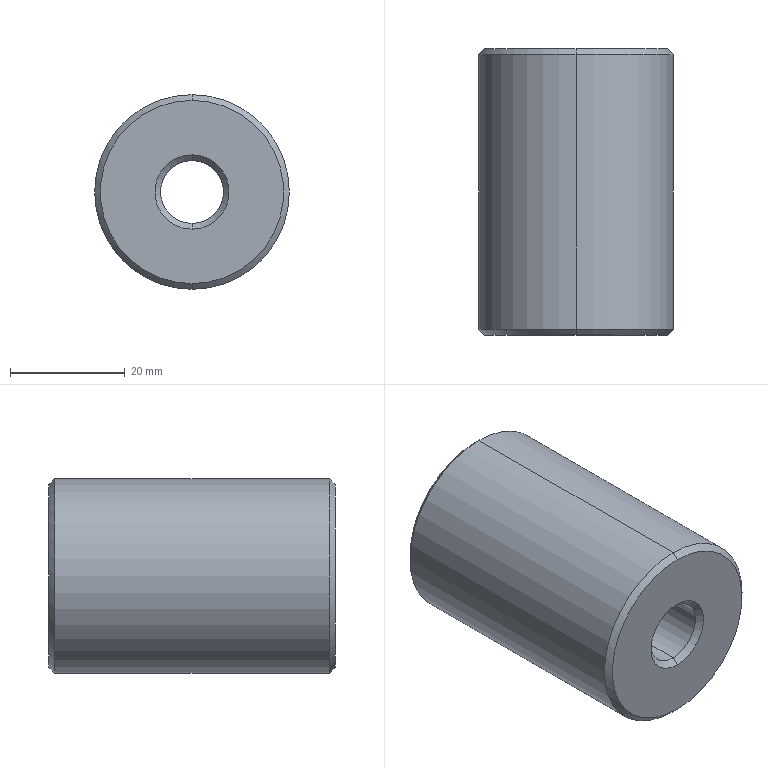Part | STEP file | Mould foot - Tower - 1 cav | 1 solid | 19 faces | box 34 x 50 x 34 mm | volume 31705 mm3 | cone 10 | cylinder 6 | plane 3 | commonest cylinder face diameters 11 x2 20 x2 34 x2
STEP:
#1=CARTESIAN_POINT('',(0.,0.,0.));
#2=DIRECTION('',(0.,0.,1.));
#3=DIRECTION('',(1.,0.,0.));
#4=AXIS2_PLACEMENT_3D('',#1,#2,#3);
#5=CARTESIAN_POINT('',(0.,9.,5.5));
#6=VERTEX_POINT('',#5);
#7=CARTESIAN_POINT('',(0.,10.,6.5));
#8=VERTEX_POINT('',#7);
#9=CARTESIAN_POINT('',(0.,10.,6.5));
#10=DIRECTION('',(0.,0.7071,0.7071));
#11=VECTOR('',#10,1.);
#12=LINE('',#9,#11);
#13=CARTESIAN_POINT('',(0.,10.,0.));
#14=DIRECTION('',(0.,1.,0.));
#15=DIRECTION('',(0.,0.,1.));
#16=AXIS2_PLACEMENT_3D('',#13,#14,#15);
#17=CONICAL_SURFACE('',#16,6.5,0.7854);
#18=CARTESIAN_POINT('',(6.283,0.));
#19=DIRECTION('',(0.,1.));
#20=VECTOR('',#19,1.);
#21=LINE('',#18,#20);
#22=(GEOMETRIC_REPRESENTATION_CONTEXT(2)PARAMETRIC_REPRESENTATION_CONTEXT()REPRESENTATION_CONTEXT('',''));
#23=DEFINITIONAL_REPRESENTATION('',(#21),#22);
#24=PCURVE('',#17,#23);
#25=CARTESIAN_POINT('',(0.,10.,0.));
#26=DIRECTION('',(0.,1.,0.));
#27=DIRECTION('',(0.,0.,1.));
#28=AXIS2_PLACEMENT_3D('',#25,#26,#27);
#29=CONICAL_SURFACE('',#28,6.5,0.7854);
#30=CARTESIAN_POINT('',(0.,0.));
#31=DIRECTION('',(0.,1.));
#32=VECTOR('',#31,1.);
#33=LINE('',#30,#32);
#34=(GEOMETRIC_REPRESENTATION_CONTEXT(2)PARAMETRIC_REPRESENTATION_CONTEXT()REPRESENTATION_CONTEXT('',''));
#35=DEFINITIONAL_REPRESENTATION('',(#33),#34);
#36=PCURVE('',#29,#35);
#37=SURFACE_CURVE('',#12,(#24,#36),.PCURVE_S1.);
#38=EDGE_CURVE('',#6,#8,#37,.T.);
#39=ORIENTED_EDGE('',*,*,#38,.T.);
#40=CARTESIAN_POINT('',(0.,10.,-6.5));
#41=VERTEX_POINT('',#40);
#42=CARTESIAN_POINT('',(0.,10.,0.));
#43=DIRECTION('',(0.,-1.,0.));
#44=DIRECTION('',(0.,0.,-1.));
#45=AXIS2_PLACEMENT_3D('',#42,#43,#44);
#46=CIRCLE('',#45,6.5);
#47=CARTESIAN_POINT('',(9.425,0.));
#48=DIRECTION('',(-1.,0.));
#49=VECTOR('',#48,1.);
#50=LINE('',#47,#49);
#51=(GEOMETRIC_REPRESENTATION_CONTEXT(2)PARAMETRIC_REPRESENTATION_CONTEXT()REPRESENTATION_CONTEXT('',''));
#52=DEFINITIONAL_REPRESENTATION('',(#50),#51);
#53=PCURVE('',#17,#52);
#54=CARTESIAN_POINT('',(0.,10.,-6.5));
#55=DIRECTION('',(0.,1.,0.));
#56=DIRECTION('',(0.,0.,1.));
#57=AXIS2_PLACEMENT_3D('',#54,#55,#56);
#58=PLANE('',#57);
#59=CARTESIAN_POINT('',(0.,0.));
#60=CARTESIAN_POINT('',(0.,11.258));
#61=CARTESIAN_POINT('',(9.75,5.629));
#62=CARTESIAN_POINT('',(19.5,0.));
#63=CARTESIAN_POINT('',(9.75,-5.629));
#64=CARTESIAN_POINT('',(0.,-11.258));
#65=CARTESIAN_POINT('',(0.,0.));
#66=(BOUNDED_CURVE()B_SPLINE_CURVE(2,(#59,#60,#61,#62,#63,#64,#65),.UNSPECIFIED.,.T.,.F.)B_SPLINE_CURVE_WITH_KNOTS((1,2,2,2,2,1),(-2.094,0.,2.094,4.189,6.283,8.378),.UNSPECIFIED.)CURVE()GEOMETRIC_REPRESENTATION_ITEM()RATIONAL_B_SPLINE_CURVE((1.,0.5,1.,0.5,1.,0.5,1.))REPRESENTATION_ITEM(''));
#67=(GEOMETRIC_REPRESENTATION_CONTEXT(2)PARAMETRIC_REPRESENTATION_CONTEXT()REPRESENTATION_CONTEXT('',''));
#68=DEFINITIONAL_REPRESENTATION('',(#66),#67);
#69=PCURVE('',#58,#68);
#70=SURFACE_CURVE('',#46,(#53,#69),.PCURVE_S1.);
#71=EDGE_CURVE('',#8,#41,#70,.T.);
#72=ORIENTED_EDGE('',*,*,#71,.T.);
#73=CARTESIAN_POINT('',(0.,9.,-5.5));
#74=VERTEX_POINT('',#73);
#75=CARTESIAN_POINT('',(0.,10.,-6.5));
#76=DIRECTION('',(0.,0.7071,-0.7071));
#77=VECTOR('',#76,1.);
#78=LINE('',#75,#77);
#79=CARTESIAN_POINT('',(3.142,0.));
#80=DIRECTION('',(0.,1.));
#81=VECTOR('',#80,1.);
#82=LINE('',#79,#81);
#83=(GEOMETRIC_REPRESENTATION_CONTEXT(2)PARAMETRIC_REPRESENTATION_CONTEXT()REPRESENTATION_CONTEXT('',''));
#84=DEFINITIONAL_REPRESENTATION('',(#82),#83);
#85=PCURVE('',#17,#84);
#86=CARTESIAN_POINT('',(3.142,0.));
#87=DIRECTION('',(0.,1.));
#88=VECTOR('',#87,1.);
#89=LINE('',#86,#88);
#90=(GEOMETRIC_REPRESENTATION_CONTEXT(2)PARAMETRIC_REPRESENTATION_CONTEXT()REPRESENTATION_CONTEXT('',''));
#91=DEFINITIONAL_REPRESENTATION('',(#89),#90);
#92=PCURVE('',#29,#91);
#93=SURFACE_CURVE('',#78,(#85,#92),.PCURVE_S1.);
#94=EDGE_CURVE('',#74,#41,#93,.T.);
#95=ORIENTED_EDGE('',*,*,#94,.F.);
#96=CARTESIAN_POINT('',(0.,9.,0.));
#97=DIRECTION('',(0.,-1.,0.));
#98=DIRECTION('',(0.,0.,-1.));
#99=AXIS2_PLACEMENT_3D('',#96,#97,#98);
#100=CIRCLE('',#99,5.5);
#101=CARTESIAN_POINT('',(9.425,-1.));
#102=DIRECTION('',(-1.,0.));
#103=VECTOR('',#102,1.);
#104=LINE('',#101,#103);
#105=(GEOMETRIC_REPRESENTATION_CONTEXT(2)PARAMETRIC_REPRESENTATION_CONTEXT()REPRESENTATION_CONTEXT('',''));
#106=DEFINITIONAL_REPRESENTATION('',(#104),#105);
#107=PCURVE('',#17,#106);
#108=CARTESIAN_POINT('',(0.,0.,0.));
#109=DIRECTION('',(0.,-1.,0.));
#110=DIRECTION('',(0.,0.,-1.));
#111=AXIS2_PLACEMENT_3D('',#108,#109,#110);
#112=CYLINDRICAL_SURFACE('',#111,5.5);
#113=CARTESIAN_POINT('',(0.,-9.));
#114=DIRECTION('',(1.,0.));
#115=VECTOR('',#114,1.);
#116=LINE('',#113,#115);
#117=(GEOMETRIC_REPRESENTATION_CONTEXT(2)PARAMETRIC_REPRESENTATION_CONTEXT()REPRESENTATION_CONTEXT('',''));
#118=DEFINITIONAL_REPRESENTATION('',(#116),#117);
#119=PCURVE('',#112,#118);
#120=SURFACE_CURVE('',#100,(#107,#119),.PCURVE_S1.);
#121=EDGE_CURVE('',#6,#74,#120,.T.);
#122=ORIENTED_EDGE('',*,*,#121,.F.);
#123=EDGE_LOOP('',(#39,#72,#95,#122));
#124=FACE_BOUND('',#123,.F.);
#125=ADVANCED_FACE('',(#124),#17,.F.);
#126=CARTESIAN_POINT('',(0.,1.,-5.5));
#127=VERTEX_POINT('',#126);
#128=CARTESIAN_POINT('',(0.,0.,-5.5));
#129=DIRECTION('',(0.,-1.,0.));
#130=VECTOR('',#129,1.);
#131=LINE('',#128,#130);
#132=CARTESIAN_POINT('',(6.283,0.));
#133=DIRECTION('',(0.,1.));
#134=VECTOR('',#133,1.);
#135=LINE('',#132,#134);
#136=(GEOMETRIC_REPRESENTATION_CONTEXT(2)PARAMETRIC_REPRESENTATION_CONTEXT()REPRESENTATION_CONTEXT('',''));
#137=DEFINITIONAL_REPRESENTATION('',(#135),#136);
#138=PCURVE('',#112,#137);
#139=CARTESIAN_POINT('',(0.,0.,0.));
#140=DIRECTION('',(0.,-1.,0.));
#141=DIRECTION('',(0.,0.,-1.));
#142=AXIS2_PLACEMENT_3D('',#139,#140,#141);
#143=CYLINDRICAL_SURFACE('',#142,5.5);
#144=CARTESIAN_POINT('',(0.,0.));
#145=DIRECTION('',(0.,1.));
#146=VECTOR('',#145,1.);
#147=LINE('',#144,#146);
#148=(GEOMETRIC_REPRESENTATION_CONTEXT(2)PARAMETRIC_REPRESENTATION_CONTEXT()REPRESENTATION_CONTEXT('',''));
#149=DEFINITIONAL_REPRESENTATION('',(#147),#148);
#150=PCURVE('',#143,#149);
#151=SURFACE_CURVE('',#131,(#138,#150),.PCURVE_S1.);
#152=EDGE_CURVE('',#74,#127,#151,.T.);
#153=ORIENTED_EDGE('',*,*,#152,.T.);
#154=CARTESIAN_POINT('',(0.,1.,5.5));
#155=VERTEX_POINT('',#154);
#156=CARTESIAN_POINT('',(0.,1.,0.));
#157=DIRECTION('',(0.,-1.,0.));
#158=DIRECTION('',(0.,0.,-1.));
#159=AXIS2_PLACEMENT_3D('',#156,#157,#158);
#160=CIRCLE('',#159,5.5);
#161=CARTESIAN_POINT('',(0.,-1.));
#162=DIRECTION('',(1.,0.));
#163=VECTOR('',#162,1.);
#164=LINE('',#161,#163);
#165=(GEOMETRIC_REPRESENTATION_CONTEXT(2)PARAMETRIC_REPRESENTATION_CONTEXT()REPRESENTATION_CONTEXT('',''));
#166=DEFINITIONAL_REPRESENTATION('',(#164),#165);
#167=PCURVE('',#112,#166);
#168=CARTESIAN_POINT('',(0.,1.,0.));
#169=DIRECTION('',(0.,-1.,0.));
#170=DIRECTION('',(0.,0.,-1.));
#171=AXIS2_PLACEMENT_3D('',#168,#169,#170);
#172=CONICAL_SURFACE('',#171,5.5,0.7854);
#173=CARTESIAN_POINT('',(0.,0.));
#174=DIRECTION('',(1.,0.));
#175=VECTOR('',#174,1.);
#176=LINE('',#173,#175);
#177=(GEOMETRIC_REPRESENTATION_CONTEXT(2)PARAMETRIC_REPRESENTATION_CONTEXT()REPRESENTATION_CONTEXT('',''));
#178=DEFINITIONAL_REPRESENTATION('',(#176),#177);
#179=PCURVE('',#172,#178);
#180=SURFACE_CURVE('',#160,(#167,#179),.PCURVE_S1.);
#181=EDGE_CURVE('',#155,#127,#180,.T.);
#182=ORIENTED_EDGE('',*,*,#181,.F.);
#183=CARTESIAN_POINT('',(0.,0.,5.5));
#184=DIRECTION('',(0.,-1.,0.));
#185=VECTOR('',#184,1.);
#186=LINE('',#183,#185);
#187=CARTESIAN_POINT('',(3.142,0.));
#188=DIRECTION('',(0.,1.));
#189=VECTOR('',#188,1.);
#190=LINE('',#187,#189);
#191=(GEOMETRIC_REPRESENTATION_CONTEXT(2)PARAMETRIC_REPRESENTATION_CONTEXT()REPRESENTATION_CONTEXT('',''));
#192=DEFINITIONAL_REPRESENTATION('',(#190),#191);
#193=PCURVE('',#112,#192);
#194=CARTESIAN_POINT('',(3.142,0.));
#195=DIRECTION('',(0.,1.));
#196=VECTOR('',#195,1.);
#197=LINE('',#194,#196);
#198=(GEOMETRIC_REPRESENTATION_CONTEXT(2)PARAMETRIC_REPRESENTATION_CONTEXT()REPRESENTATION_CONTEXT('',''));
#199=DEFINITIONAL_REPRESENTATION('',(#197),#198);
#200=PCURVE('',#143,#199);
#201=SURFACE_CURVE('',#186,(#193,#200),.PCURVE_S1.);
#202=EDGE_CURVE('',#6,#155,#201,.T.);
#203=ORIENTED_EDGE('',*,*,#202,.F.);
#204=ORIENTED_EDGE('',*,*,#121,.T.);
#205=EDGE_LOOP('',(#153,#182,#203,#204));
#206=FACE_BOUND('',#205,.F.);
#207=ADVANCED_FACE('',(#206),#112,.F.);
#208=CARTESIAN_POINT('',(0.,0.,-6.5));
#209=VERTEX_POINT('',#208);
#210=CARTESIAN_POINT('',(0.,1.,-5.5));
#211=DIRECTION('',(0.,-0.7071,-0.7071));
#212=VECTOR('',#211,1.);
#213=LINE('',#210,#212);
#214=CARTESIAN_POINT('',(6.283,0.));
#215=DIRECTION('',(0.,1.));
#216=VECTOR('',#215,1.);
#217=LINE('',#214,#216);
#218=(GEOMETRIC_REPRESENTATION_CONTEXT(2)PARAMETRIC_REPRESENTATION_CONTEXT()REPRESENTATION_CONTEXT('',''));
#219=DEFINITIONAL_REPRESENTATION('',(#217),#218);
#220=PCURVE('',#172,#219);
#221=CARTESIAN_POINT('',(0.,1.,0.));
#222=DIRECTION('',(0.,-1.,0.));
#223=DIRECTION('',(0.,0.,-1.));
#224=AXIS2_PLACEMENT_3D('',#221,#222,#223);
#225=CONICAL_SURFACE('',#224,5.5,0.7854);
#226=CARTESIAN_POINT('',(0.,0.));
#227=DIRECTION('',(0.,1.));
#228=VECTOR('',#227,1.);
#229=LINE('',#226,#228);
#230=(GEOMETRIC_REPRESENTATION_CONTEXT(2)PARAMETRIC_REPRESENTATION_CONTEXT()REPRESENTATION_CONTEXT('',''));
#231=DEFINITIONAL_REPRESENTATION('',(#229),#230);
#232=PCURVE('',#225,#231);
#233=SURFACE_CURVE('',#213,(#220,#232),.PCURVE_S1.);
#234=EDGE_CURVE('',#127,#209,#233,.T.);
#235=ORIENTED_EDGE('',*,*,#234,.T.);
#236=CARTESIAN_POINT('',(0.,0.,6.5));
#237=VERTEX_POINT('',#236);
#238=CARTESIAN_POINT('',(0.,0.,0.));
#239=DIRECTION('',(0.,-1.,0.));
#240=DIRECTION('',(0.,0.,-1.));
#241=AXIS2_PLACEMENT_3D('',#238,#239,#240);
#242=CIRCLE('',#241,6.5);
#243=CARTESIAN_POINT('',(0.,1.));
#244=DIRECTION('',(1.,0.));
#245=VECTOR('',#244,1.);
#246=LINE('',#243,#245);
#247=(GEOMETRIC_REPRESENTATION_CONTEXT(2)PARAMETRIC_REPRESENTATION_CONTEXT()REPRESENTATION_CONTEXT('',''));
#248=DEFINITIONAL_REPRESENTATION('',(#246),#247);
#249=PCURVE('',#172,#248);
#250=CARTESIAN_POINT('',(0.,0.,-16.));
#251=DIRECTION('',(0.,-1.,0.));
#252=DIRECTION('',(0.,0.,-1.));
#253=AXIS2_PLACEMENT_3D('',#250,#251,#252);
#254=PLANE('',#253);
#255=CARTESIAN_POINT('',(-16.,0.));
#256=DIRECTION('',(1.,0.));
#257=AXIS2_PLACEMENT_2D('',#255,#256);
#258=CIRCLE('',#257,6.5);
#259=(GEOMETRIC_REPRESENTATION_CONTEXT(2)PARAMETRIC_REPRESENTATION_CONTEXT()REPRESENTATION_CONTEXT('',''));
#260=DEFINITIONAL_REPRESENTATION('',(#258),#259);
#261=PCURVE('',#254,#260);
#262=SURFACE_CURVE('',#242,(#249,#261),.PCURVE_S1.);
#263=EDGE_CURVE('',#237,#209,#262,.T.);
#264=ORIENTED_EDGE('',*,*,#263,.F.);
#265=CARTESIAN_POINT('',(0.,1.,5.5));
#266=DIRECTION('',(0.,-0.7071,0.7071));
#267=VECTOR('',#266,1.);
#268=LINE('',#265,#267);
#269=CARTESIAN_POINT('',(3.142,0.));
#270=DIRECTION('',(0.,1.));
#271=VECTOR('',#270,1.);
#272=LINE('',#269,#271);
#273=(GEOMETRIC_REPRESENTATION_CONTEXT(2)PARAMETRIC_REPRESENTATION_CONTEXT()REPRESENTATION_CONTEXT('',''));
#274=DEFINITIONAL_REPRESENTATION('',(#272),#273);
#275=PCURVE('',#172,#274);
#276=CARTESIAN_POINT('',(3.142,0.));
#277=DIRECTION('',(0.,1.));
#278=VECTOR('',#277,1.);
#279=LINE('',#276,#278);
#280=(GEOMETRIC_REPRESENTATION_CONTEXT(2)PARAMETRIC_REPRESENTATION_CONTEXT()REPRESENTATION_CONTEXT('',''));
#281=DEFINITIONAL_REPRESENTATION('',(#279),#280);
#282=PCURVE('',#225,#281);
#283=SURFACE_CURVE('',#268,(#275,#282),.PCURVE_S1.);
#284=EDGE_CURVE('',#155,#237,#283,.T.);
#285=ORIENTED_EDGE('',*,*,#284,.F.);
#286=ORIENTED_EDGE('',*,*,#181,.T.);
#287=EDGE_LOOP('',(#235,#264,#285,#286));
#288=FACE_BOUND('',#287,.F.);
#289=ADVANCED_FACE('',(#288),#172,.F.);
#290=CARTESIAN_POINT('',(0.,0.,-16.));
#291=VERTEX_POINT('',#290);
#292=CARTESIAN_POINT('',(0.,0.,16.));
#293=VERTEX_POINT('',#292);
#294=CARTESIAN_POINT('',(0.,0.,0.));
#295=DIRECTION('',(0.,-1.,0.));
#296=DIRECTION('',(0.,0.,-1.));
#297=AXIS2_PLACEMENT_3D('',#294,#295,#296);
#298=CIRCLE('',#297,16.);
#299=CARTESIAN_POINT('',(0.,0.,0.));
#300=DIRECTION('',(0.,1.,0.));
#301=DIRECTION('',(0.,0.,1.));
#302=AXIS2_PLACEMENT_3D('',#299,#300,#301);
#303=CONICAL_SURFACE('',#302,16.,0.7854);
#304=CARTESIAN_POINT('',(3.142,0.));
#305=DIRECTION('',(-1.,0.));
#306=VECTOR('',#305,1.);
#307=LINE('',#304,#306);
#308=(GEOMETRIC_REPRESENTATION_CONTEXT(2)PARAMETRIC_REPRESENTATION_CONTEXT()REPRESENTATION_CONTEXT('',''));
#309=DEFINITIONAL_REPRESENTATION('',(#307),#308);
#310=PCURVE('',#303,#309);
#311=CARTESIAN_POINT('',(-16.,0.));
#312=DIRECTION('',(1.,0.));
#313=AXIS2_PLACEMENT_2D('',#311,#312);
#314=CIRCLE('',#313,16.);
#315=(GEOMETRIC_REPRESENTATION_CONTEXT(2)PARAMETRIC_REPRESENTATION_CONTEXT()REPRESENTATION_CONTEXT('',''));
#316=DEFINITIONAL_REPRESENTATION('',(#314),#315);
#317=PCURVE('',#254,#316);
#318=SURFACE_CURVE('',#298,(#310,#317),.PCURVE_S1.);
#319=EDGE_CURVE('',#291,#293,#318,.T.);
#320=ORIENTED_EDGE('',*,*,#319,.F.);
#321=CARTESIAN_POINT('',(0.,1.,-17.));
#322=VERTEX_POINT('',#321);
#323=CARTESIAN_POINT('',(0.,0.,-16.));
#324=DIRECTION('',(0.,0.7071,-0.7071));
#325=VECTOR('',#324,1.);
#326=LINE('',#323,#325);
#327=CARTESIAN_POINT('',(3.142,0.));
#328=DIRECTION('',(0.,1.));
#329=VECTOR('',#328,1.);
#330=LINE('',#327,#329);
#331=(GEOMETRIC_REPRESENTATION_CONTEXT(2)PARAMETRIC_REPRESENTATION_CONTEXT()REPRESENTATION_CONTEXT('',''));
#332=DEFINITIONAL_REPRESENTATION('',(#330),#331);
#333=PCURVE('',#303,#332);
#334=CARTESIAN_POINT('',(0.,0.,0.));
#335=DIRECTION('',(0.,1.,0.));
#336=DIRECTION('',(0.,0.,1.));
#337=AXIS2_PLACEMENT_3D('',#334,#335,#336);
#338=CONICAL_SURFACE('',#337,16.,0.7854);
#339=CARTESIAN_POINT('',(3.142,0.));
#340=DIRECTION('',(0.,1.));
#341=VECTOR('',#340,1.);
#342=LINE('',#339,#341);
#343=(GEOMETRIC_REPRESENTATION_CONTEXT(2)PARAMETRIC_REPRESENTATION_CONTEXT()REPRESENTATION_CONTEXT('',''));
#344=DEFINITIONAL_REPRESENTATION('',(#342),#343);
#345=PCURVE('',#338,#344);
#346=SURFACE_CURVE('',#326,(#333,#345),.PCURVE_S1.);
#347=EDGE_CURVE('',#291,#322,#346,.T.);
#348=ORIENTED_EDGE('',*,*,#347,.T.);
#349=CARTESIAN_POINT('',(0.,1.,17.));
#350=VERTEX_POINT('',#349);
#351=CARTESIAN_POINT('',(0.,1.,0.));
#352=DIRECTION('',(0.,-1.,0.));
#353=DIRECTION('',(0.,0.,-1.));
#354=AXIS2_PLACEMENT_3D('',#351,#352,#353);
#355=CIRCLE('',#354,17.);
#356=CARTESIAN_POINT('',(3.142,1.));
#357=DIRECTION('',(-1.,0.));
#358=VECTOR('',#357,1.);
#359=LINE('',#356,#358);
#360=(GEOMETRIC_REPRESENTATION_CONTEXT(2)PARAMETRIC_REPRESENTATION_CONTEXT()REPRESENTATION_CONTEXT('',''));
#361=DEFINITIONAL_REPRESENTATION('',(#359),#360);
#362=PCURVE('',#303,#361);
#363=CARTESIAN_POINT('',(0.,0.,0.));
#364=DIRECTION('',(0.,-1.,0.));
#365=DIRECTION('',(0.,0.,-1.));
#366=AXIS2_PLACEMENT_3D('',#363,#364,#365);
#367=CYLINDRICAL_SURFACE('',#366,17.);
#368=CARTESIAN_POINT('',(0.,-1.));
#369=DIRECTION('',(1.,0.));
#370=VECTOR('',#369,1.);
#371=LINE('',#368,#370);
#372=(GEOMETRIC_REPRESENTATION_CONTEXT(2)PARAMETRIC_REPRESENTATION_CONTEXT()REPRESENTATION_CONTEXT('',''));
#373=DEFINITIONAL_REPRESENTATION('',(#371),#372);
#374=PCURVE('',#367,#373);
#375=SURFACE_CURVE('',#355,(#362,#374),.PCURVE_S1.);
#376=EDGE_CURVE('',#322,#350,#375,.T.);
#377=ORIENTED_EDGE('',*,*,#376,.T.);
#378=CARTESIAN_POINT('',(0.,0.,16.));
#379=DIRECTION('',(0.,0.7071,0.7071));
#380=VECTOR('',#379,1.);
#381=LINE('',#378,#380);
#382=CARTESIAN_POINT('',(0.,0.));
#383=DIRECTION('',(0.,1.));
#384=VECTOR('',#383,1.);
#385=LINE('',#382,#384);
#386=(GEOMETRIC_REPRESENTATION_CONTEXT(2)PARAMETRIC_REPRESENTATION_CONTEXT()REPRESENTATION_CONTEXT('',''));
#387=DEFINITIONAL_REPRESENTATION('',(#385),#386);
#388=PCURVE('',#303,#387);
#389=CARTESIAN_POINT('',(6.283,0.));
#390=DIRECTION('',(0.,1.));
#391=VECTOR('',#390,1.);
#392=LINE('',#389,#391);
#393=(GEOMETRIC_REPRESENTATION_CONTEXT(2)PARAMETRIC_REPRESENTATION_CONTEXT()REPRESENTATION_CONTEXT('',''));
#394=DEFINITIONAL_REPRESENTATION('',(#392),#393);
#395=PCURVE('',#338,#394);
#396=SURFACE_CURVE('',#381,(#388,#395),.PCURVE_S1.);
#397=EDGE_CURVE('',#293,#350,#396,.T.);
#398=ORIENTED_EDGE('',*,*,#397,.F.);
#399=EDGE_LOOP('',(#320,#348,#377,#398));
#400=FACE_BOUND('',#399,.T.);
#401=ADVANCED_FACE('',(#400),#303,.T.);
#402=CARTESIAN_POINT('',(0.,49.,-17.));
#403=VERTEX_POINT('',#402);
#404=CARTESIAN_POINT('',(0.,49.,17.));
#405=VERTEX_POINT('',#404);
#406=CARTESIAN_POINT('',(0.,49.,0.));
#407=DIRECTION('',(0.,-1.,0.));
#408=DIRECTION('',(0.,0.,-1.));
#409=AXIS2_PLACEMENT_3D('',#406,#407,#408);
#410=CIRCLE('',#409,17.);
#411=CARTESIAN_POINT('',(0.,-49.));
#412=DIRECTION('',(1.,0.));
#413=VECTOR('',#412,1.);
#414=LINE('',#411,#413);
#415=(GEOMETRIC_REPRESENTATION_CONTEXT(2)PARAMETRIC_REPRESENTATION_CONTEXT()REPRESENTATION_CONTEXT('',''));
#416=DEFINITIONAL_REPRESENTATION('',(#414),#415);
#417=PCURVE('',#367,#416);
#418=CARTESIAN_POINT('',(0.,49.,0.));
#419=DIRECTION('',(0.,-1.,0.));
#420=DIRECTION('',(0.,0.,-1.));
#421=AXIS2_PLACEMENT_3D('',#418,#419,#420);
#422=CONICAL_SURFACE('',#421,17.,0.7854);
#423=CARTESIAN_POINT('',(0.,0.));
#424=DIRECTION('',(1.,0.));
#425=VECTOR('',#424,1.);
#426=LINE('',#423,#425);
#427=(GEOMETRIC_REPRESENTATION_CONTEXT(2)PARAMETRIC_REPRESENTATION_CONTEXT()REPRESENTATION_CONTEXT('',''));
#428=DEFINITIONAL_REPRESENTATION('',(#426),#427);
#429=PCURVE('',#422,#428);
#430=SURFACE_CURVE('',#410,(#417,#429),.PCURVE_S1.);
#431=EDGE_CURVE('',#403,#405,#430,.T.);
#432=ORIENTED_EDGE('',*,*,#431,.T.);
#433=CARTESIAN_POINT('',(0.,0.,17.));
#434=DIRECTION('',(0.,-1.,0.));
#435=VECTOR('',#434,1.);
#436=LINE('',#433,#435);
#437=CARTESIAN_POINT('',(3.142,0.));
#438=DIRECTION('',(0.,1.));
#439=VECTOR('',#438,1.);
#440=LINE('',#437,#439);
#441=(GEOMETRIC_REPRESENTATION_CONTEXT(2)PARAMETRIC_REPRESENTATION_CONTEXT()REPRESENTATION_CONTEXT('',''));
#442=DEFINITIONAL_REPRESENTATION('',(#440),#441);
#443=PCURVE('',#367,#442);
#444=CARTESIAN_POINT('',(0.,0.,0.));
#445=DIRECTION('',(0.,-1.,0.));
#446=DIRECTION('',(0.,0.,-1.));
#447=AXIS2_PLACEMENT_3D('',#444,#445,#446);
#448=CYLINDRICAL_SURFACE('',#447,17.);
#449=CARTESIAN_POINT('',(3.142,0.));
#450=DIRECTION('',(0.,1.));
#451=VECTOR('',#450,1.);
#452=LINE('',#449,#451);
#453=(GEOMETRIC_REPRESENTATION_CONTEXT(2)PARAMETRIC_REPRESENTATION_CONTEXT()REPRESENTATION_CONTEXT('',''));
#454=DEFINITIONAL_REPRESENTATION('',(#452),#453);
#455=PCURVE('',#448,#454);
#456=SURFACE_CURVE('',#436,(#443,#455),.PCURVE_S1.);
#457=EDGE_CURVE('',#405,#350,#456,.T.);
#458=ORIENTED_EDGE('',*,*,#457,.T.);
#459=ORIENTED_EDGE('',*,*,#376,.F.);
#460=CARTESIAN_POINT('',(0.,0.,-17.));
#461=DIRECTION('',(0.,-1.,0.));
#462=VECTOR('',#461,1.);
#463=LINE('',#460,#462);
#464=CARTESIAN_POINT('',(0.,0.));
#465=DIRECTION('',(0.,1.));
#466=VECTOR('',#465,1.);
#467=LINE('',#464,#466);
#468=(GEOMETRIC_REPRESENTATION_CONTEXT(2)PARAMETRIC_REPRESENTATION_CONTEXT()REPRESENTATION_CONTEXT('',''));
#469=DEFINITIONAL_REPRESENTATION('',(#467),#468);
#470=PCURVE('',#367,#469);
#471=CARTESIAN_POINT('',(6.283,0.));
#472=DIRECTION('',(0.,1.));
#473=VECTOR('',#472,1.);
#474=LINE('',#471,#473);
#475=(GEOMETRIC_REPRESENTATION_CONTEXT(2)PARAMETRIC_REPRESENTATION_CONTEXT()REPRESENTATION_CONTEXT('',''));
#476=DEFINITIONAL_REPRESENTATION('',(#474),#475);
#477=PCURVE('',#448,#476);
#478=SURFACE_CURVE('',#463,(#470,#477),.PCURVE_S1.);
#479=EDGE_CURVE('',#403,#322,#478,.T.);
#480=ORIENTED_EDGE('',*,*,#479,.F.);
#481=EDGE_LOOP('',(#432,#458,#459,#480));
#482=FACE_BOUND('',#481,.T.);
#483=ADVANCED_FACE('',(#482),#367,.T.);
#484=CARTESIAN_POINT('',(0.,50.,-16.));
#485=VERTEX_POINT('',#484);
#486=CARTESIAN_POINT('',(0.,50.,16.));
#487=VERTEX_POINT('',#486);
#488=CARTESIAN_POINT('',(0.,50.,0.));
#489=DIRECTION('',(0.,-1.,0.));
#490=DIRECTION('',(0.,0.,-1.));
#491=AXIS2_PLACEMENT_3D('',#488,#489,#490);
#492=CIRCLE('',#491,16.);
#493=CARTESIAN_POINT('',(0.,-1.));
#494=DIRECTION('',(1.,0.));
#495=VECTOR('',#494,1.);
#496=LINE('',#493,#495);
#497=(GEOMETRIC_REPRESENTATION_CONTEXT(2)PARAMETRIC_REPRESENTATION_CONTEXT()REPRESENTATION_CONTEXT('',''));
#498=DEFINITIONAL_REPRESENTATION('',(#496),#497);
#499=PCURVE('',#422,#498);
#500=CARTESIAN_POINT('',(0.,50.,-11.));
#501=DIRECTION('',(0.,1.,0.));
#502=DIRECTION('',(0.,0.,1.));
#503=AXIS2_PLACEMENT_3D('',#500,#501,#502);
#504=PLANE('',#503);
#505=CARTESIAN_POINT('',(-5.,0.));
#506=CARTESIAN_POINT('',(-5.,27.713));
#507=CARTESIAN_POINT('',(19.,13.856));
#508=CARTESIAN_POINT('',(43.,0.));
#509=CARTESIAN_POINT('',(19.,-13.856));
#510=CARTESIAN_POINT('',(-5.,-27.713));
#511=CARTESIAN_POINT('',(-5.,0.));
#512=(BOUNDED_CURVE()B_SPLINE_CURVE(2,(#505,#506,#507,#508,#509,#510,#511),.UNSPECIFIED.,.T.,.F.)B_SPLINE_CURVE_WITH_KNOTS((1,2,2,2,2,1),(-2.094,0.,2.094,4.189,6.283,8.378),.UNSPECIFIED.)CURVE()GEOMETRIC_REPRESENTATION_ITEM()RATIONAL_B_SPLINE_CURVE((1.,0.5,1.,0.5,1.,0.5,1.))REPRESENTATION_ITEM(''));
#513=(GEOMETRIC_REPRESENTATION_CONTEXT(2)PARAMETRIC_REPRESENTATION_CONTEXT()REPRESENTATION_CONTEXT('',''));
#514=DEFINITIONAL_REPRESENTATION('',(#512),#513);
#515=PCURVE('',#504,#514);
#516=SURFACE_CURVE('',#492,(#499,#515),.PCURVE_S1.);
#517=EDGE_CURVE('',#485,#487,#516,.T.);
#518=ORIENTED_EDGE('',*,*,#517,.T.);
#519=CARTESIAN_POINT('',(0.,49.,17.));
#520=DIRECTION('',(0.,-0.7071,0.7071));
#521=VECTOR('',#520,1.);
#522=LINE('',#519,#521);
#523=CARTESIAN_POINT('',(3.142,0.));
#524=DIRECTION('',(0.,1.));
#525=VECTOR('',#524,1.);
#526=LINE('',#523,#525);
#527=(GEOMETRIC_REPRESENTATION_CONTEXT(2)PARAMETRIC_REPRESENTATION_CONTEXT()REPRESENTATION_CONTEXT('',''));
#528=DEFINITIONAL_REPRESENTATION('',(#526),#527);
#529=PCURVE('',#422,#528);
#530=CARTESIAN_POINT('',(0.,49.,0.));
#531=DIRECTION('',(0.,-1.,0.));
#532=DIRECTION('',(0.,0.,-1.));
#533=AXIS2_PLACEMENT_3D('',#530,#531,#532);
#534=CONICAL_SURFACE('',#533,17.,0.7854);
#535=CARTESIAN_POINT('',(3.142,0.));
#536=DIRECTION('',(0.,1.));
#537=VECTOR('',#536,1.);
#538=LINE('',#535,#537);
#539=(GEOMETRIC_REPRESENTATION_CONTEXT(2)PARAMETRIC_REPRESENTATION_CONTEXT()REPRESENTATION_CONTEXT('',''));
#540=DEFINITIONAL_REPRESENTATION('',(#538),#539);
#541=PCURVE('',#534,#540);
#542=SURFACE_CURVE('',#522,(#529,#541),.PCURVE_S1.);
#543=EDGE_CURVE('',#487,#405,#542,.T.);
#544=ORIENTED_EDGE('',*,*,#543,.T.);
#545=ORIENTED_EDGE('',*,*,#431,.F.);
#546=CARTESIAN_POINT('',(0.,49.,-17.));
#547=DIRECTION('',(0.,-0.7071,-0.7071));
#548=VECTOR('',#547,1.);
#549=LINE('',#546,#548);
#550=CARTESIAN_POINT('',(0.,0.));
#551=DIRECTION('',(0.,1.));
#552=VECTOR('',#551,1.);
#553=LINE('',#550,#552);
#554=(GEOMETRIC_REPRESENTATION_CONTEXT(2)PARAMETRIC_REPRESENTATION_CONTEXT()REPRESENTATION_CONTEXT('',''));
#555=DEFINITIONAL_REPRESENTATION('',(#553),#554);
#556=PCURVE('',#422,#555);
#557=CARTESIAN_POINT('',(6.283,0.));
#558=DIRECTION('',(0.,1.));
#559=VECTOR('',#558,1.);
#560=LINE('',#557,#559);
#561=(GEOMETRIC_REPRESENTATION_CONTEXT(2)PARAMETRIC_REPRESENTATION_CONTEXT()REPRESENTATION_CONTEXT('',''));
#562=DEFINITIONAL_REPRESENTATION('',(#560),#561);
#563=PCURVE('',#534,#562);
#564=SURFACE_CURVE('',#549,(#556,#563),.PCURVE_S1.);
#565=EDGE_CURVE('',#485,#403,#564,.T.);
#566=ORIENTED_EDGE('',*,*,#565,.F.);
#567=EDGE_LOOP('',(#518,#544,#545,#566));
#568=FACE_BOUND('',#567,.T.);
#569=ADVANCED_FACE('',(#568),#422,.T.);
#570=CARTESIAN_POINT('',(0.,49.,10.));
#571=VERTEX_POINT('',#570);
#572=CARTESIAN_POINT('',(0.,50.,11.));
#573=VERTEX_POINT('',#572);
#574=CARTESIAN_POINT('',(0.,50.,11.));
#575=DIRECTION('',(0.,0.7071,0.7071));
#576=VECTOR('',#575,1.);
#577=LINE('',#574,#576);
#578=CARTESIAN_POINT('',(0.,50.,0.));
#579=DIRECTION('',(0.,1.,0.));
#580=DIRECTION('',(0.,0.,1.));
#581=AXIS2_PLACEMENT_3D('',#578,#579,#580);
#582=CONICAL_SURFACE('',#581,11.,0.7854);
#583=CARTESIAN_POINT('',(6.283,0.));
#584=DIRECTION('',(0.,1.));
#585=VECTOR('',#584,1.);
#586=LINE('',#583,#585);
#587=(GEOMETRIC_REPRESENTATION_CONTEXT(2)PARAMETRIC_REPRESENTATION_CONTEXT()REPRESENTATION_CONTEXT('',''));
#588=DEFINITIONAL_REPRESENTATION('',(#586),#587);
#589=PCURVE('',#582,#588);
#590=CARTESIAN_POINT('',(0.,50.,0.));
#591=DIRECTION('',(0.,1.,0.));
#592=DIRECTION('',(0.,0.,1.));
#593=AXIS2_PLACEMENT_3D('',#590,#591,#592);
#594=CONICAL_SURFACE('',#593,11.,0.7854);
#595=CARTESIAN_POINT('',(0.,0.));
#596=DIRECTION('',(0.,1.));
#597=VECTOR('',#596,1.);
#598=LINE('',#595,#597);
#599=(GEOMETRIC_REPRESENTATION_CONTEXT(2)PARAMETRIC_REPRESENTATION_CONTEXT()REPRESENTATION_CONTEXT('',''));
#600=DEFINITIONAL_REPRESENTATION('',(#598),#599);
#601=PCURVE('',#594,#600);
#602=SURFACE_CURVE('',#577,(#589,#601),.PCURVE_S1.);
#603=EDGE_CURVE('',#571,#573,#602,.T.);
#604=ORIENTED_EDGE('',*,*,#603,.T.);
#605=CARTESIAN_POINT('',(0.,50.,-11.));
#606=VERTEX_POINT('',#605);
#607=CARTESIAN_POINT('',(0.,50.,0.));
#608=DIRECTION('',(0.,-1.,0.));
#609=DIRECTION('',(0.,0.,-1.));
#610=AXIS2_PLACEMENT_3D('',#607,#608,#609);
#611=CIRCLE('',#610,11.);
#612=CARTESIAN_POINT('',(9.425,0.));
#613=DIRECTION('',(-1.,0.));
#614=VECTOR('',#613,1.);
#615=LINE('',#612,#614);
#616=(GEOMETRIC_REPRESENTATION_CONTEXT(2)PARAMETRIC_REPRESENTATION_CONTEXT()REPRESENTATION_CONTEXT('',''));
#617=DEFINITIONAL_REPRESENTATION('',(#615),#616);
#618=PCURVE('',#582,#617);
#619=CARTESIAN_POINT('',(0.,0.));
#620=CARTESIAN_POINT('',(0.,19.053));
#621=CARTESIAN_POINT('',(16.5,9.526));
#622=CARTESIAN_POINT('',(33.,0.));
#623=CARTESIAN_POINT('',(16.5,-9.526));
#624=CARTESIAN_POINT('',(0.,-19.053));
#625=CARTESIAN_POINT('',(0.,0.));
#626=(BOUNDED_CURVE()B_SPLINE_CURVE(2,(#619,#620,#621,#622,#623,#624,#625),.UNSPECIFIED.,.T.,.F.)B_SPLINE_CURVE_WITH_KNOTS((1,2,2,2,2,1),(-2.094,0.,2.094,4.189,6.283,8.378),.UNSPECIFIED.)CURVE()GEOMETRIC_REPRESENTATION_ITEM()RATIONAL_B_SPLINE_CURVE((1.,0.5,1.,0.5,1.,0.5,1.))REPRESENTATION_ITEM(''));
#627=(GEOMETRIC_REPRESENTATION_CONTEXT(2)PARAMETRIC_REPRESENTATION_CONTEXT()REPRESENTATION_CONTEXT('',''));
#628=DEFINITIONAL_REPRESENTATION('',(#626),#627);
#629=PCURVE('',#504,#628);
#630=SURFACE_CURVE('',#611,(#618,#629),.PCURVE_S1.);
#631=EDGE_CURVE('',#573,#606,#630,.T.);
#632=ORIENTED_EDGE('',*,*,#631,.T.);
#633=CARTESIAN_POINT('',(0.,49.,-10.));
#634=VERTEX_POINT('',#633);
#635=CARTESIAN_POINT('',(0.,50.,-11.));
#636=DIRECTION('',(0.,0.7071,-0.7071));
#637=VECTOR('',#636,1.);
#638=LINE('',#635,#637);
#639=CARTESIAN_POINT('',(3.142,0.));
#640=DIRECTION('',(0.,1.));
#641=VECTOR('',#640,1.);
#642=LINE('',#639,#641);
#643=(GEOMETRIC_REPRESENTATION_CONTEXT(2)PARAMETRIC_REPRESENTATION_CONTEXT()REPRESENTATION_CONTEXT('',''));
#644=DEFINITIONAL_REPRESENTATION('',(#642),#643);
#645=PCURVE('',#582,#644);
#646=CARTESIAN_POINT('',(3.142,0.));
#647=DIRECTION('',(0.,1.));
#648=VECTOR('',#647,1.);
#649=LINE('',#646,#648);
#650=(GEOMETRIC_REPRESENTATION_CONTEXT(2)PARAMETRIC_REPRESENTATION_CONTEXT()REPRESENTATION_CONTEXT('',''));
#651=DEFINITIONAL_REPRESENTATION('',(#649),#650);
#652=PCURVE('',#594,#651);
#653=SURFACE_CURVE('',#638,(#645,#652),.PCURVE_S1.);
#654=EDGE_CURVE('',#634,#606,#653,.T.);
#655=ORIENTED_EDGE('',*,*,#654,.F.);
#656=CARTESIAN_POINT('',(0.,49.,0.));
#657=DIRECTION('',(0.,-1.,0.));
#658=DIRECTION('',(0.,0.,-1.));
#659=AXIS2_PLACEMENT_3D('',#656,#657,#658);
#660=CIRCLE('',#659,10.);
#661=CARTESIAN_POINT('',(9.425,-1.));
#662=DIRECTION('',(-1.,0.));
#663=VECTOR('',#662,1.);
#664=LINE('',#661,#663);
#665=(GEOMETRIC_REPRESENTATION_CONTEXT(2)PARAMETRIC_REPRESENTATION_CONTEXT()REPRESENTATION_CONTEXT('',''));
#666=DEFINITIONAL_REPRESENTATION('',(#664),#665);
#667=PCURVE('',#582,#666);
#668=CARTESIAN_POINT('',(0.,0.,0.));
#669=DIRECTION('',(0.,-1.,0.));
#670=DIRECTION('',(0.,0.,-1.));
#671=AXIS2_PLACEMENT_3D('',#668,#669,#670);
#672=CYLINDRICAL_SURFACE('',#671,10.);
#673=CARTESIAN_POINT('',(0.,-49.));
#674=DIRECTION('',(1.,0.));
#675=VECTOR('',#674,1.);
#676=LINE('',#673,#675);
#677=(GEOMETRIC_REPRESENTATION_CONTEXT(2)PARAMETRIC_REPRESENTATION_CONTEXT()REPRESENTATION_CONTEXT('',''));
#678=DEFINITIONAL_REPRESENTATION('',(#676),#677);
#679=PCURVE('',#672,#678);
#680=SURFACE_CURVE('',#660,(#667,#679),.PCURVE_S1.);
#681=EDGE_CURVE('',#571,#634,#680,.T.);
#682=ORIENTED_EDGE('',*,*,#681,.F.);
#683=EDGE_LOOP('',(#604,#632,#655,#682));
#684=FACE_BOUND('',#683,.F.);
#685=ADVANCED_FACE('',(#684),#582,.F.);
#686=CARTESIAN_POINT('',(0.,10.,-10.));
#687=VERTEX_POINT('',#686);
#688=CARTESIAN_POINT('',(0.,0.,-10.));
#689=DIRECTION('',(0.,-1.,0.));
#690=VECTOR('',#689,1.);
#691=LINE('',#688,#690);
#692=CARTESIAN_POINT('',(6.283,0.));
#693=DIRECTION('',(0.,1.));
#694=VECTOR('',#693,1.);
#695=LINE('',#692,#694);
#696=(GEOMETRIC_REPRESENTATION_CONTEXT(2)PARAMETRIC_REPRESENTATION_CONTEXT()REPRESENTATION_CONTEXT('',''));
#697=DEFINITIONAL_REPRESENTATION('',(#695),#696);
#698=PCURVE('',#672,#697);
#699=CARTESIAN_POINT('',(0.,0.,0.));
#700=DIRECTION('',(0.,-1.,0.));
#701=DIRECTION('',(0.,0.,-1.));
#702=AXIS2_PLACEMENT_3D('',#699,#700,#701);
#703=CYLINDRICAL_SURFACE('',#702,10.);
#704=CARTESIAN_POINT('',(0.,0.));
#705=DIRECTION('',(0.,1.));
#706=VECTOR('',#705,1.);
#707=LINE('',#704,#706);
#708=(GEOMETRIC_REPRESENTATION_CONTEXT(2)PARAMETRIC_REPRESENTATION_CONTEXT()REPRESENTATION_CONTEXT('',''));
#709=DEFINITIONAL_REPRESENTATION('',(#707),#708);
#710=PCURVE('',#703,#709);
#711=SURFACE_CURVE('',#691,(#698,#710),.PCURVE_S1.);
#712=EDGE_CURVE('',#634,#687,#711,.T.);
#713=ORIENTED_EDGE('',*,*,#712,.T.);
#714=CARTESIAN_POINT('',(0.,10.,10.));
#715=VERTEX_POINT('',#714);
#716=CARTESIAN_POINT('',(0.,10.,0.));
#717=DIRECTION('',(0.,-1.,0.));
#718=DIRECTION('',(0.,0.,-1.));
#719=AXIS2_PLACEMENT_3D('',#716,#717,#718);
#720=CIRCLE('',#719,10.);
#721=CARTESIAN_POINT('',(0.,-10.));
#722=DIRECTION('',(1.,0.));
#723=VECTOR('',#722,1.);
#724=LINE('',#721,#723);
#725=(GEOMETRIC_REPRESENTATION_CONTEXT(2)PARAMETRIC_REPRESENTATION_CONTEXT()REPRESENTATION_CONTEXT('',''));
#726=DEFINITIONAL_REPRESENTATION('',(#724),#725);
#727=PCURVE('',#672,#726);
#728=CARTESIAN_POINT('',(-3.5,0.));
#729=CARTESIAN_POINT('',(-3.5,17.321));
#730=CARTESIAN_POINT('',(11.5,8.66));
#731=CARTESIAN_POINT('',(26.5,0.));
#732=CARTESIAN_POINT('',(11.5,-8.66));
#733=CARTESIAN_POINT('',(-3.5,-17.321));
#734=CARTESIAN_POINT('',(-3.5,0.));
#735=(BOUNDED_CURVE()B_SPLINE_CURVE(2,(#728,#729,#730,#731,#732,#733,#734),.UNSPECIFIED.,.T.,.F.)B_SPLINE_CURVE_WITH_KNOTS((1,2,2,2,2,1),(-2.094,0.,2.094,4.189,6.283,8.378),.UNSPECIFIED.)CURVE()GEOMETRIC_REPRESENTATION_ITEM()RATIONAL_B_SPLINE_CURVE((1.,0.5,1.,0.5,1.,0.5,1.))REPRESENTATION_ITEM(''));
#736=(GEOMETRIC_REPRESENTATION_CONTEXT(2)PARAMETRIC_REPRESENTATION_CONTEXT()REPRESENTATION_CONTEXT('',''));
#737=DEFINITIONAL_REPRESENTATION('',(#735),#736);
#738=PCURVE('',#58,#737);
#739=SURFACE_CURVE('',#720,(#727,#738),.PCURVE_S1.);
#740=EDGE_CURVE('',#715,#687,#739,.T.);
#741=ORIENTED_EDGE('',*,*,#740,.F.);
#742=CARTESIAN_POINT('',(0.,0.,10.));
#743=DIRECTION('',(0.,-1.,0.));
#744=VECTOR('',#743,1.);
#745=LINE('',#742,#744);
#746=CARTESIAN_POINT('',(3.142,0.));
#747=DIRECTION('',(0.,1.));
#748=VECTOR('',#747,1.);
#749=LINE('',#746,#748);
#750=(GEOMETRIC_REPRESENTATION_CONTEXT(2)PARAMETRIC_REPRESENTATION_CONTEXT()REPRESENTATION_CONTEXT('',''));
#751=DEFINITIONAL_REPRESENTATION('',(#749),#750);
#752=PCURVE('',#672,#751);
#753=CARTESIAN_POINT('',(3.142,0.));
#754=DIRECTION('',(0.,1.));
#755=VECTOR('',#754,1.);
#756=LINE('',#753,#755);
#757=(GEOMETRIC_REPRESENTATION_CONTEXT(2)PARAMETRIC_REPRESENTATION_CONTEXT()REPRESENTATION_CONTEXT('',''));
#758=DEFINITIONAL_REPRESENTATION('',(#756),#757);
#759=PCURVE('',#703,#758);
#760=SURFACE_CURVE('',#745,(#752,#759),.PCURVE_S1.);
#761=EDGE_CURVE('',#571,#715,#760,.T.);
#762=ORIENTED_EDGE('',*,*,#761,.F.);
#763=ORIENTED_EDGE('',*,*,#681,.T.);
#764=EDGE_LOOP('',(#713,#741,#762,#763));
#765=FACE_BOUND('',#764,.F.);
#766=ADVANCED_FACE('',(#765),#672,.F.);
#767=CARTESIAN_POINT('',(0.,10.,0.));
#768=DIRECTION('',(0.,-1.,0.));
#769=DIRECTION('',(0.,0.,-1.));
#770=AXIS2_PLACEMENT_3D('',#767,#768,#769);
#771=CIRCLE('',#770,10.);
#772=CARTESIAN_POINT('',(0.,-10.));
#773=DIRECTION('',(1.,0.));
#774=VECTOR('',#773,1.);
#775=LINE('',#772,#774);
#776=(GEOMETRIC_REPRESENTATION_CONTEXT(2)PARAMETRIC_REPRESENTATION_CONTEXT()REPRESENTATION_CONTEXT('',''));
#777=DEFINITIONAL_REPRESENTATION('',(#775),#776);
#778=PCURVE('',#703,#777);
#779=CARTESIAN_POINT('',(-3.5,0.));
#780=CARTESIAN_POINT('',(-3.5,17.321));
#781=CARTESIAN_POINT('',(11.5,8.66));
#782=CARTESIAN_POINT('',(26.5,0.));
#783=CARTESIAN_POINT('',(11.5,-8.66));
#784=CARTESIAN_POINT('',(-3.5,-17.321));
#785=CARTESIAN_POINT('',(-3.5,0.));
#786=(BOUNDED_CURVE()B_SPLINE_CURVE(2,(#779,#780,#781,#782,#783,#784,#785),.UNSPECIFIED.,.T.,.F.)B_SPLINE_CURVE_WITH_KNOTS((1,2,2,2,2,1),(-2.094,0.,2.094,4.189,6.283,8.378),.UNSPECIFIED.)CURVE()GEOMETRIC_REPRESENTATION_ITEM()RATIONAL_B_SPLINE_CURVE((1.,0.5,1.,0.5,1.,0.5,1.))REPRESENTATION_ITEM(''));
#787=(GEOMETRIC_REPRESENTATION_CONTEXT(2)PARAMETRIC_REPRESENTATION_CONTEXT()REPRESENTATION_CONTEXT('',''));
#788=DEFINITIONAL_REPRESENTATION('',(#786),#787);
#789=PCURVE('',#58,#788);
#790=SURFACE_CURVE('',#771,(#778,#789),.PCURVE_S1.);
#791=EDGE_CURVE('',#687,#715,#790,.T.);
#792=ORIENTED_EDGE('',*,*,#791,.F.);
#793=ORIENTED_EDGE('',*,*,#712,.F.);
#794=CARTESIAN_POINT('',(0.,49.,0.));
#795=DIRECTION('',(0.,-1.,0.));
#796=DIRECTION('',(0.,0.,-1.));
#797=AXIS2_PLACEMENT_3D('',#794,#795,#796);
#798=CIRCLE('',#797,10.);
#799=CARTESIAN_POINT('',(0.,-49.));
#800=DIRECTION('',(1.,0.));
#801=VECTOR('',#800,1.);
#802=LINE('',#799,#801);
#803=(GEOMETRIC_REPRESENTATION_CONTEXT(2)PARAMETRIC_REPRESENTATION_CONTEXT()REPRESENTATION_CONTEXT('',''));
#804=DEFINITIONAL_REPRESENTATION('',(#802),#803);
#805=PCURVE('',#703,#804);
#806=CARTESIAN_POINT('',(3.142,-1.));
#807=DIRECTION('',(-1.,0.));
#808=VECTOR('',#807,1.);
#809=LINE('',#806,#808);
#810=(GEOMETRIC_REPRESENTATION_CONTEXT(2)PARAMETRIC_REPRESENTATION_CONTEXT()REPRESENTATION_CONTEXT('',''));
#811=DEFINITIONAL_REPRESENTATION('',(#809),#810);
#812=PCURVE('',#594,#811);
#813=SURFACE_CURVE('',#798,(#805,#812),.PCURVE_S1.);
#814=EDGE_CURVE('',#634,#571,#813,.T.);
#815=ORIENTED_EDGE('',*,*,#814,.T.);
#816=ORIENTED_EDGE('',*,*,#761,.T.);
#817=EDGE_LOOP('',(#792,#793,#815,#816));
#818=FACE_BOUND('',#817,.F.);
#819=ADVANCED_FACE('',(#818),#703,.F.);
#820=CARTESIAN_POINT('',(0.,50.,0.));
#821=DIRECTION('',(0.,-1.,0.));
#822=DIRECTION('',(0.,0.,-1.));
#823=AXIS2_PLACEMENT_3D('',#820,#821,#822);
#824=CIRCLE('',#823,11.);
#825=CARTESIAN_POINT('',(3.142,0.));
#826=DIRECTION('',(-1.,0.));
#827=VECTOR('',#826,1.);
#828=LINE('',#825,#827);
#829=(GEOMETRIC_REPRESENTATION_CONTEXT(2)PARAMETRIC_REPRESENTATION_CONTEXT()REPRESENTATION_CONTEXT('',''));
#830=DEFINITIONAL_REPRESENTATION('',(#828),#829);
#831=PCURVE('',#594,#830);
#832=CARTESIAN_POINT('',(0.,0.));
#833=CARTESIAN_POINT('',(0.,19.053));
#834=CARTESIAN_POINT('',(16.5,9.526));
#835=CARTESIAN_POINT('',(33.,0.));
#836=CARTESIAN_POINT('',(16.5,-9.526));
#837=CARTESIAN_POINT('',(0.,-19.053));
#838=CARTESIAN_POINT('',(0.,0.));
#839=(BOUNDED_CURVE()B_SPLINE_CURVE(2,(#832,#833,#834,#835,#836,#837,#838),.UNSPECIFIED.,.T.,.F.)B_SPLINE_CURVE_WITH_KNOTS((1,2,2,2,2,1),(-2.094,0.,2.094,4.189,6.283,8.378),.UNSPECIFIED.)CURVE()GEOMETRIC_REPRESENTATION_ITEM()RATIONAL_B_SPLINE_CURVE((1.,0.5,1.,0.5,1.,0.5,1.))REPRESENTATION_ITEM(''));
#840=(GEOMETRIC_REPRESENTATION_CONTEXT(2)PARAMETRIC_REPRESENTATION_CONTEXT()REPRESENTATION_CONTEXT('',''));
#841=DEFINITIONAL_REPRESENTATION('',(#839),#840);
#842=PCURVE('',#504,#841);
#843=SURFACE_CURVE('',#824,(#831,#842),.PCURVE_S1.);
#844=EDGE_CURVE('',#606,#573,#843,.T.);
#845=ORIENTED_EDGE('',*,*,#844,.T.);
#846=ORIENTED_EDGE('',*,*,#603,.F.);
#847=ORIENTED_EDGE('',*,*,#814,.F.);
#848=ORIENTED_EDGE('',*,*,#654,.T.);
#849=EDGE_LOOP('',(#845,#846,#847,#848));
#850=FACE_BOUND('',#849,.F.);
#851=ADVANCED_FACE('',(#850),#594,.F.);
#852=ORIENTED_EDGE('',*,*,#631,.T.);
#853=ORIENTED_EDGE('',*,*,#844,.T.);
#854=EDGE_LOOP('',(#852,#853));
#855=FACE_BOUND('',#854,.T.);
#856=ORIENTED_EDGE('',*,*,#517,.F.);
#857=CARTESIAN_POINT('',(0.,50.,0.));
#858=DIRECTION('',(0.,-1.,0.));
#859=DIRECTION('',(0.,0.,-1.));
#860=AXIS2_PLACEMENT_3D('',#857,#858,#859);
#861=CIRCLE('',#860,16.);
#862=CARTESIAN_POINT('',(-5.,0.));
#863=CARTESIAN_POINT('',(-5.,27.713));
#864=CARTESIAN_POINT('',(19.,13.856));
#865=CARTESIAN_POINT('',(43.,0.));
#866=CARTESIAN_POINT('',(19.,-13.856));
#867=CARTESIAN_POINT('',(-5.,-27.713));
#868=CARTESIAN_POINT('',(-5.,0.));
#869=(BOUNDED_CURVE()B_SPLINE_CURVE(2,(#862,#863,#864,#865,#866,#867,#868),.UNSPECIFIED.,.T.,.F.)B_SPLINE_CURVE_WITH_KNOTS((1,2,2,2,2,1),(-2.094,0.,2.094,4.189,6.283,8.378),.UNSPECIFIED.)CURVE()GEOMETRIC_REPRESENTATION_ITEM()RATIONAL_B_SPLINE_CURVE((1.,0.5,1.,0.5,1.,0.5,1.))REPRESENTATION_ITEM(''));
#870=(GEOMETRIC_REPRESENTATION_CONTEXT(2)PARAMETRIC_REPRESENTATION_CONTEXT()REPRESENTATION_CONTEXT('',''));
#871=DEFINITIONAL_REPRESENTATION('',(#869),#870);
#872=PCURVE('',#504,#871);
#873=CARTESIAN_POINT('',(0.,-1.));
#874=DIRECTION('',(1.,0.));
#875=VECTOR('',#874,1.);
#876=LINE('',#873,#875);
#877=(GEOMETRIC_REPRESENTATION_CONTEXT(2)PARAMETRIC_REPRESENTATION_CONTEXT()REPRESENTATION_CONTEXT('',''));
#878=DEFINITIONAL_REPRESENTATION('',(#876),#877);
#879=PCURVE('',#534,#878);
#880=SURFACE_CURVE('',#861,(#872,#879),.PCURVE_S1.);
#881=EDGE_CURVE('',#487,#485,#880,.T.);
#882=ORIENTED_EDGE('',*,*,#881,.F.);
#883=EDGE_LOOP('',(#856,#882));
#884=FACE_BOUND('',#883,.T.);
#885=ADVANCED_FACE('',(#855,#884),#504,.T.);
#886=ORIENTED_EDGE('',*,*,#543,.F.);
#887=ORIENTED_EDGE('',*,*,#881,.T.);
#888=ORIENTED_EDGE('',*,*,#565,.T.);
#889=CARTESIAN_POINT('',(0.,49.,0.));
#890=DIRECTION('',(0.,-1.,0.));
#891=DIRECTION('',(0.,0.,-1.));
#892=AXIS2_PLACEMENT_3D('',#889,#890,#891);
#893=CIRCLE('',#892,17.);
#894=CARTESIAN_POINT('',(0.,0.));
#895=DIRECTION('',(1.,0.));
#896=VECTOR('',#895,1.);
#897=LINE('',#894,#896);
#898=(GEOMETRIC_REPRESENTATION_CONTEXT(2)PARAMETRIC_REPRESENTATION_CONTEXT()REPRESENTATION_CONTEXT('',''));
#899=DEFINITIONAL_REPRESENTATION('',(#897),#898);
#900=PCURVE('',#534,#899);
#901=CARTESIAN_POINT('',(0.,-49.));
#902=DIRECTION('',(1.,0.));
#903=VECTOR('',#902,1.);
#904=LINE('',#901,#903);
#905=(GEOMETRIC_REPRESENTATION_CONTEXT(2)PARAMETRIC_REPRESENTATION_CONTEXT()REPRESENTATION_CONTEXT('',''));
#906=DEFINITIONAL_REPRESENTATION('',(#904),#905);
#907=PCURVE('',#448,#906);
#908=SURFACE_CURVE('',#893,(#900,#907),.PCURVE_S1.);
#909=EDGE_CURVE('',#405,#403,#908,.T.);
#910=ORIENTED_EDGE('',*,*,#909,.F.);
#911=EDGE_LOOP('',(#886,#887,#888,#910));
#912=FACE_BOUND('',#911,.T.);
#913=ADVANCED_FACE('',(#912),#534,.T.);
#914=ORIENTED_EDGE('',*,*,#457,.F.);
#915=ORIENTED_EDGE('',*,*,#909,.T.);
#916=ORIENTED_EDGE('',*,*,#479,.T.);
#917=CARTESIAN_POINT('',(0.,1.,0.));
#918=DIRECTION('',(0.,-1.,0.));
#919=DIRECTION('',(0.,0.,-1.));
#920=AXIS2_PLACEMENT_3D('',#917,#918,#919);
#921=CIRCLE('',#920,17.);
#922=CARTESIAN_POINT('',(0.,-1.));
#923=DIRECTION('',(1.,0.));
#924=VECTOR('',#923,1.);
#925=LINE('',#922,#924);
#926=(GEOMETRIC_REPRESENTATION_CONTEXT(2)PARAMETRIC_REPRESENTATION_CONTEXT()REPRESENTATION_CONTEXT('',''));
#927=DEFINITIONAL_REPRESENTATION('',(#925),#926);
#928=PCURVE('',#448,#927);
#929=CARTESIAN_POINT('',(9.425,1.));
#930=DIRECTION('',(-1.,0.));
#931=VECTOR('',#930,1.);
#932=LINE('',#929,#931);
#933=(GEOMETRIC_REPRESENTATION_CONTEXT(2)PARAMETRIC_REPRESENTATION_CONTEXT()REPRESENTATION_CONTEXT('',''));
#934=DEFINITIONAL_REPRESENTATION('',(#932),#933);
#935=PCURVE('',#338,#934);
#936=SURFACE_CURVE('',#921,(#928,#935),.PCURVE_S1.);
#937=EDGE_CURVE('',#350,#322,#936,.T.);
#938=ORIENTED_EDGE('',*,*,#937,.F.);
#939=EDGE_LOOP('',(#914,#915,#916,#938));
#940=FACE_BOUND('',#939,.T.);
#941=ADVANCED_FACE('',(#940),#448,.T.);
#942=ORIENTED_EDGE('',*,*,#347,.F.);
#943=CARTESIAN_POINT('',(0.,0.,0.));
#944=DIRECTION('',(0.,-1.,0.));
#945=DIRECTION('',(0.,0.,-1.));
#946=AXIS2_PLACEMENT_3D('',#943,#944,#945);
#947=CIRCLE('',#946,16.);
#948=CARTESIAN_POINT('',(9.425,0.));
#949=DIRECTION('',(-1.,0.));
#950=VECTOR('',#949,1.);
#951=LINE('',#948,#950);
#952=(GEOMETRIC_REPRESENTATION_CONTEXT(2)PARAMETRIC_REPRESENTATION_CONTEXT()REPRESENTATION_CONTEXT('',''));
#953=DEFINITIONAL_REPRESENTATION('',(#951),#952);
#954=PCURVE('',#338,#953);
#955=CARTESIAN_POINT('',(-16.,0.));
#956=DIRECTION('',(1.,0.));
#957=AXIS2_PLACEMENT_2D('',#955,#956);
#958=CIRCLE('',#957,16.);
#959=(GEOMETRIC_REPRESENTATION_CONTEXT(2)PARAMETRIC_REPRESENTATION_CONTEXT()REPRESENTATION_CONTEXT('',''));
#960=DEFINITIONAL_REPRESENTATION('',(#958),#959);
#961=PCURVE('',#254,#960);
#962=SURFACE_CURVE('',#947,(#954,#961),.PCURVE_S1.);
#963=EDGE_CURVE('',#293,#291,#962,.T.);
#964=ORIENTED_EDGE('',*,*,#963,.F.);
#965=ORIENTED_EDGE('',*,*,#397,.T.);
#966=ORIENTED_EDGE('',*,*,#937,.T.);
#967=EDGE_LOOP('',(#942,#964,#965,#966));
#968=FACE_BOUND('',#967,.T.);
#969=ADVANCED_FACE('',(#968),#338,.T.);
#970=ORIENTED_EDGE('',*,*,#963,.T.);
#971=ORIENTED_EDGE('',*,*,#319,.T.);
#972=EDGE_LOOP('',(#970,#971));
#973=FACE_BOUND('',#972,.T.);
#974=CARTESIAN_POINT('',(0.,0.,0.));
#975=DIRECTION('',(0.,-1.,0.));
#976=DIRECTION('',(0.,0.,-1.));
#977=AXIS2_PLACEMENT_3D('',#974,#975,#976);
#978=CIRCLE('',#977,6.5);
#979=CARTESIAN_POINT('',(-16.,0.));
#980=DIRECTION('',(1.,0.));
#981=AXIS2_PLACEMENT_2D('',#979,#980);
#982=CIRCLE('',#981,6.5);
#983=(GEOMETRIC_REPRESENTATION_CONTEXT(2)PARAMETRIC_REPRESENTATION_CONTEXT()REPRESENTATION_CONTEXT('',''));
#984=DEFINITIONAL_REPRESENTATION('',(#982),#983);
#985=PCURVE('',#254,#984);
#986=CARTESIAN_POINT('',(0.,1.));
#987=DIRECTION('',(1.,0.));
#988=VECTOR('',#987,1.);
#989=LINE('',#986,#988);
#990=(GEOMETRIC_REPRESENTATION_CONTEXT(2)PARAMETRIC_REPRESENTATION_CONTEXT()REPRESENTATION_CONTEXT('',''));
#991=DEFINITIONAL_REPRESENTATION('',(#989),#990);
#992=PCURVE('',#225,#991);
#993=SURFACE_CURVE('',#978,(#985,#992),.PCURVE_S1.);
#994=EDGE_CURVE('',#209,#237,#993,.T.);
#995=ORIENTED_EDGE('',*,*,#994,.F.);
#996=ORIENTED_EDGE('',*,*,#263,.F.);
#997=EDGE_LOOP('',(#995,#996));
#998=FACE_BOUND('',#997,.T.);
#999=ADVANCED_FACE('',(#973,#998),#254,.T.);
#1000=ORIENTED_EDGE('',*,*,#994,.F.);
#1001=ORIENTED_EDGE('',*,*,#234,.F.);
#1002=CARTESIAN_POINT('',(0.,1.,0.));
#1003=DIRECTION('',(0.,-1.,0.));
#1004=DIRECTION('',(0.,0.,-1.));
#1005=AXIS2_PLACEMENT_3D('',#1002,#1003,#1004);
#1006=CIRCLE('',#1005,5.5);
#1007=CARTESIAN_POINT('',(0.,0.));
#1008=DIRECTION('',(1.,0.));
#1009=VECTOR('',#1008,1.);
#1010=LINE('',#1007,#1009);
#1011=(GEOMETRIC_REPRESENTATION_CONTEXT(2)PARAMETRIC_REPRESENTATION_CONTEXT()REPRESENTATION_CONTEXT('',''));
#1012=DEFINITIONAL_REPRESENTATION('',(#1010),#1011);
#1013=PCURVE('',#225,#1012);
#1014=CARTESIAN_POINT('',(0.,-1.));
#1015=DIRECTION('',(1.,0.));
#1016=VECTOR('',#1015,1.);
#1017=LINE('',#1014,#1016);
#1018=(GEOMETRIC_REPRESENTATION_CONTEXT(2)PARAMETRIC_REPRESENTATION_CONTEXT()REPRESENTATION_CONTEXT('',''));
#1019=DEFINITIONAL_REPRESENTATION('',(#1017),#1018);
#1020=PCURVE('',#143,#1019);
#1021=SURFACE_CURVE('',#1006,(#1013,#1020),.PCURVE_S1.);
#1022=EDGE_CURVE('',#127,#155,#1021,.T.);
#1023=ORIENTED_EDGE('',*,*,#1022,.T.);
#1024=ORIENTED_EDGE('',*,*,#284,.T.);
#1025=EDGE_LOOP('',(#1000,#1001,#1023,#1024));
#1026=FACE_BOUND('',#1025,.F.);
#1027=ADVANCED_FACE('',(#1026),#225,.F.);
#1028=ORIENTED_EDGE('',*,*,#1022,.F.);
#1029=ORIENTED_EDGE('',*,*,#152,.F.);
#1030=CARTESIAN_POINT('',(0.,9.,0.));
#1031=DIRECTION('',(0.,-1.,0.));
#1032=DIRECTION('',(0.,0.,-1.));
#1033=AXIS2_PLACEMENT_3D('',#1030,#1031,#1032);
#1034=CIRCLE('',#1033,5.5);
#1035=CARTESIAN_POINT('',(0.,-9.));
#1036=DIRECTION('',(1.,0.));
#1037=VECTOR('',#1036,1.);
#1038=LINE('',#1035,#1037);
#1039=(GEOMETRIC_REPRESENTATION_CONTEXT(2)PARAMETRIC_REPRESENTATION_CONTEXT()REPRESENTATION_CONTEXT('',''));
#1040=DEFINITIONAL_REPRESENTATION('',(#1038),#1039);
#1041=PCURVE('',#143,#1040);
#1042=CARTESIAN_POINT('',(3.142,-1.));
#1043=DIRECTION('',(-1.,0.));
#1044=VECTOR('',#1043,1.);
#1045=LINE('',#1042,#1044);
#1046=(GEOMETRIC_REPRESENTATION_CONTEXT(2)PARAMETRIC_REPRESENTATION_CONTEXT()REPRESENTATION_CONTEXT('',''));
#1047=DEFINITIONAL_REPRESENTATION('',(#1045),#1046);
#1048=PCURVE('',#29,#1047);
#1049=SURFACE_CURVE('',#1034,(#1041,#1048),.PCURVE_S1.);
#1050=EDGE_CURVE('',#74,#6,#1049,.T.);
#1051=ORIENTED_EDGE('',*,*,#1050,.T.);
#1052=ORIENTED_EDGE('',*,*,#202,.T.);
#1053=EDGE_LOOP('',(#1028,#1029,#1051,#1052));
#1054=FACE_BOUND('',#1053,.F.);
#1055=ADVANCED_FACE('',(#1054),#143,.F.);
#1056=CARTESIAN_POINT('',(0.,10.,0.));
#1057=DIRECTION('',(0.,-1.,0.));
#1058=DIRECTION('',(0.,0.,-1.));
#1059=AXIS2_PLACEMENT_3D('',#1056,#1057,#1058);
#1060=CIRCLE('',#1059,6.5);
#1061=CARTESIAN_POINT('',(3.142,0.));
#1062=DIRECTION('',(-1.,0.));
#1063=VECTOR('',#1062,1.);
#1064=LINE('',#1061,#1063);
#1065=(GEOMETRIC_REPRESENTATION_CONTEXT(2)PARAMETRIC_REPRESENTATION_CONTEXT()REPRESENTATION_CONTEXT('',''));
#1066=DEFINITIONAL_REPRESENTATION('',(#1064),#1065);
#1067=PCURVE('',#29,#1066);
#1068=CARTESIAN_POINT('',(0.,0.));
#1069=CARTESIAN_POINT('',(0.,11.258));
#1070=CARTESIAN_POINT('',(9.75,5.629));
#1071=CARTESIAN_POINT('',(19.5,0.));
#1072=CARTESIAN_POINT('',(9.75,-5.629));
#1073=CARTESIAN_POINT('',(0.,-11.258));
#1074=CARTESIAN_POINT('',(0.,0.));
#1075=(BOUNDED_CURVE()B_SPLINE_CURVE(2,(#1068,#1069,#1070,#1071,#1072,#1073,#1074),.UNSPECIFIED.,.T.,.F.)B_SPLINE_CURVE_WITH_KNOTS((1,2,2,2,2,1),(-2.094,0.,2.094,4.189,6.283,8.378),.UNSPECIFIED.)CURVE()GEOMETRIC_REPRESENTATION_ITEM()RATIONAL_B_SPLINE_CURVE((1.,0.5,1.,0.5,1.,0.5,1.))REPRESENTATION_ITEM(''));
#1076=(GEOMETRIC_REPRESENTATION_CONTEXT(2)PARAMETRIC_REPRESENTATION_CONTEXT()REPRESENTATION_CONTEXT('',''));
#1077=DEFINITIONAL_REPRESENTATION('',(#1075),#1076);
#1078=PCURVE('',#58,#1077);
#1079=SURFACE_CURVE('',#1060,(#1067,#1078),.PCURVE_S1.);
#1080=EDGE_CURVE('',#41,#8,#1079,.T.);
#1081=ORIENTED_EDGE('',*,*,#1080,.T.);
#1082=ORIENTED_EDGE('',*,*,#38,.F.);
#1083=ORIENTED_EDGE('',*,*,#1050,.F.);
#1084=ORIENTED_EDGE('',*,*,#94,.T.);
#1085=EDGE_LOOP('',(#1081,#1082,#1083,#1084));
#1086=FACE_BOUND('',#1085,.F.);
#1087=ADVANCED_FACE('',(#1086),#29,.F.);
#1088=ORIENTED_EDGE('',*,*,#71,.T.);
#1089=ORIENTED_EDGE('',*,*,#1080,.T.);
#1090=EDGE_LOOP('',(#1088,#1089));
#1091=FACE_BOUND('',#1090,.T.);
#1092=ORIENTED_EDGE('',*,*,#791,.F.);
#1093=ORIENTED_EDGE('',*,*,#740,.F.);
#1094=EDGE_LOOP('',(#1092,#1093));
#1095=FACE_BOUND('',#1094,.T.);
#1096=ADVANCED_FACE('',(#1091,#1095),#58,.T.);
#1097=CLOSED_SHELL('',(#125,#207,#289,#401,#483,#569,#685,#766,#819,#851,#885,#913,#941,#969,#999,#1027,#1055,#1087,#1096));
#1098=MANIFOLD_SOLID_BREP('',#1097);
#1099=(LENGTH_UNIT()NAMED_UNIT(*)SI_UNIT(.MILLI.,.METRE.));
#1100=UNCERTAINTY_MEASURE_WITH_UNIT(LENGTH_MEASURE(0.0000001),#1099,'','');
#1101=(NAMED_UNIT(*)PLANE_ANGLE_UNIT()SI_UNIT($,.RADIAN.));
#1102=(NAMED_UNIT(*)SI_UNIT($,.STERADIAN.)SOLID_ANGLE_UNIT());
#1103=(GEOMETRIC_REPRESENTATION_CONTEXT(3)GLOBAL_UNCERTAINTY_ASSIGNED_CONTEXT((#1100))GLOBAL_UNIT_ASSIGNED_CONTEXT((#1099,#1101,#1102))REPRESENTATION_CONTEXT('',''));
#1104=ADVANCED_BREP_SHAPE_REPRESENTATION('',(#4,#1098),#1103);